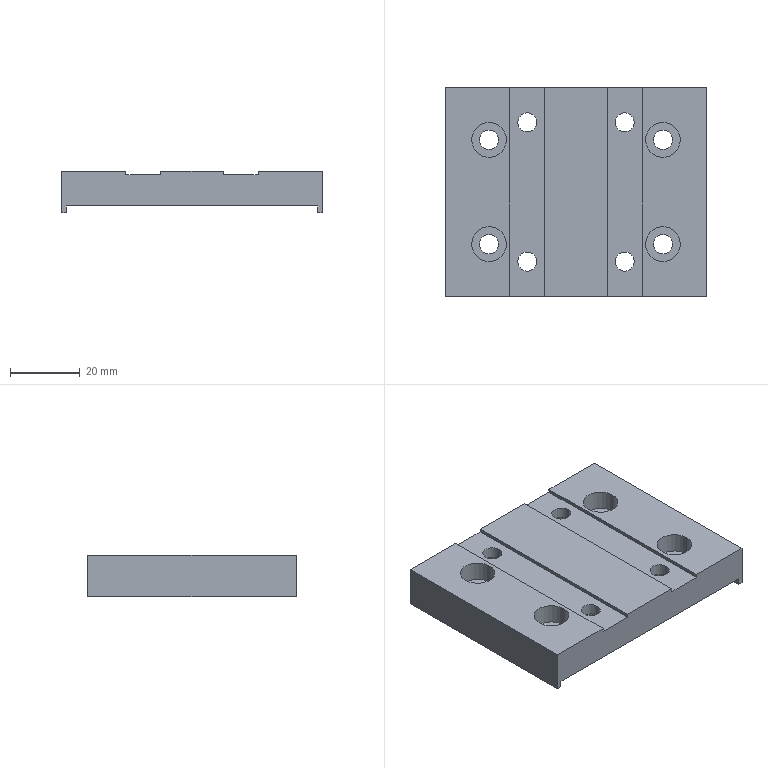Part | STEP file | PN_0089 Mount electronic clip connecting plate C | 1 solid | 58 faces | box 75 x 60 x 12 mm | volume 39832 mm3 | cylinder 32 | plane 26 | commonest cylinder face diameters 5.5 x16 10 x16